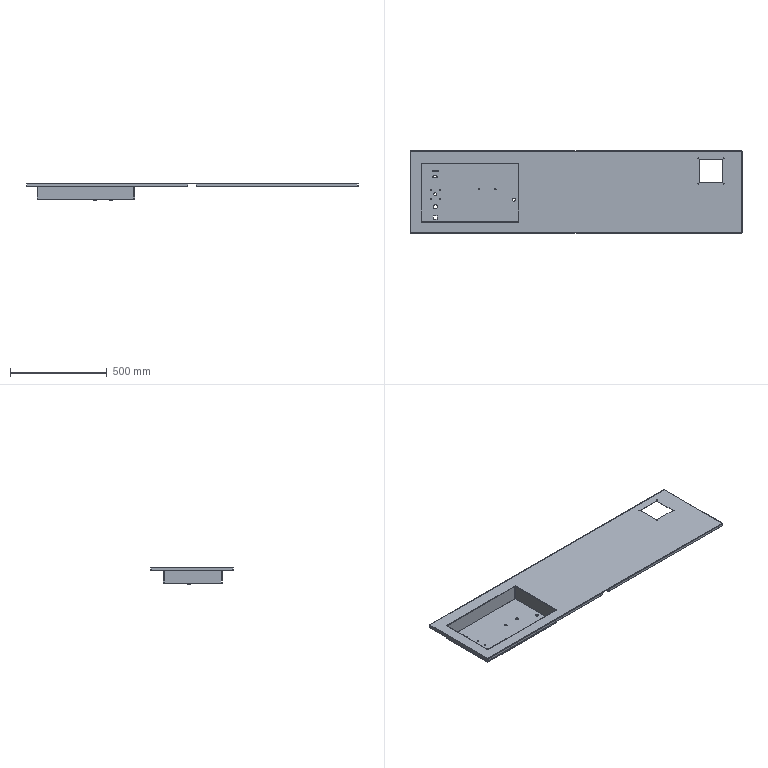Part | STEP file | 1 solid | 148 faces | box 1718 x 428 x 87.5 mm | volume 1351126 mm3 | plane 68 | cylinder 64 | spline 16 | commonest cylinder face diameters 1 x10 2 x8 3.2 x8 4 x8 4.5 x8 5.5 x8